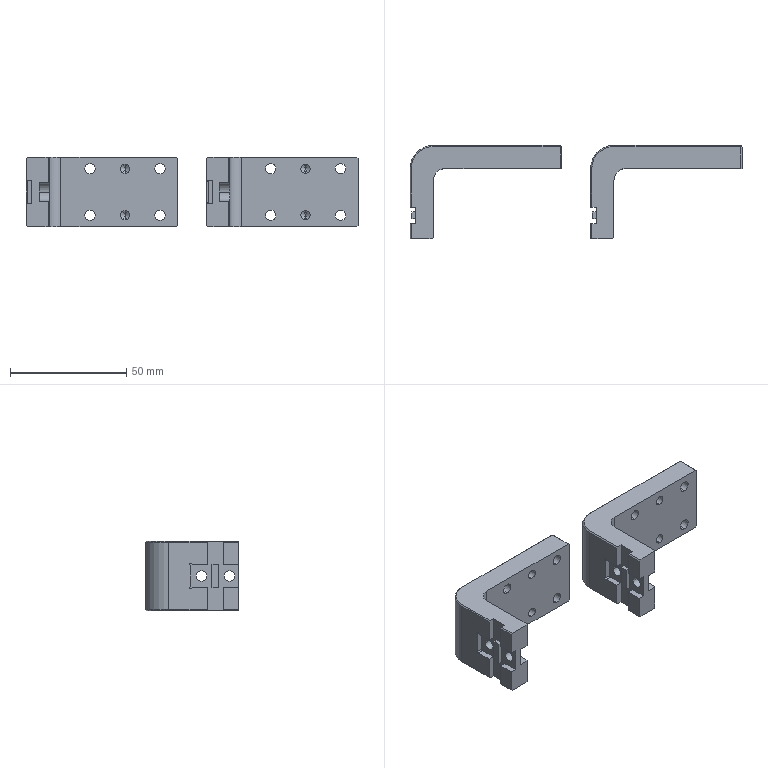NC program | NX | posted with a generic post | part box 142.5 x 40 x 30 mm
Lines 5775 to 5836 of 5836:
(PLANAR_MILL_COPY_COPY_COPY , TOOL : D6A45)
N11548 T01 M6
N11550 G17 G43 G0 G90 X-35.116 Y21.4 Z30. B0. C0. S9500 H1 M3
N11552 Z0.5
N11554 G94 G1 Z-1. F1250.
N11556 G3 X-34.25 Y20.9 R1.
N11558 G1 X-7.25
N11560 G2 X-5.35 Y19. R1.9
N11562 G1 Y10.
N11564 G2 X-6.25 Y9.1 R0.9
N11566 G1 X-56.25
N11568 G3 X-60.35 Y5. R4.1
N11570 G1 Y-19.5
N11572 G2 X-60.614 Y-20.136 R0.9
N11574 G1 X-61.114 Y-20.636
N11576 G2 X-61.75 Y-20.9 R0.9
N11578 G1 X-71.25
N11580 G2 X-72.15 Y-20. R0.9
N11582 G1 Y-13.55
N11584 G2 X-71.25 Y-12.65 R0.9
N11586 G1 X-69.65
N11588 Y-7.45
N11590 X-71.25
N11592 G2 X-72.15 Y-6.55 R0.9
N11594 G1 Y10.
N11596 G2 X-61.25 Y20.9 R10.9
N11598 G1 X-34.25
N11600 G3 X-33.384 Y21.4 R1.
N11602 G1 Z0.5
N11604 G0 Z30.
N11606 X42.384
N11608 Z0.5
N11610 G1 Z-1.
N11612 G3 X43.25 Y20.9 R1.
N11614 G1 X70.25
N11616 G2 X72.15 Y19. R1.9
N11618 G1 Y10.
N11620 G2 X71.25 Y9.1 R0.9
N11622 G1 X21.25
N11624 G3 X17.15 Y5. R4.1
N11626 G1 Y-19.5
N11628 G2 X16.886 Y-20.136 R0.9
N11630 G1 X16.386 Y-20.636
N11632 G2 X15.75 Y-20.9 R0.9
N11634 G1 X6.25
N11636 G2 X5.35 Y-20. R0.9
N11638 G1 Y-13.55
N11640 G2 X6.25 Y-12.65 R0.9
N11642 G1 X7.85
N11644 Y-7.45
N11646 X6.25
N11648 G2 X5.35 Y-6.55 R0.9
N11650 G1 Y10.
N11652 G2 X16.25 Y20.9 R10.9
N11654 G1 X43.25
N11656 G3 X44.116 Y21.4 R1.
N11658 G1 Z0.5
N11660 G0 Z30.
N11662 M5
N11664 M2